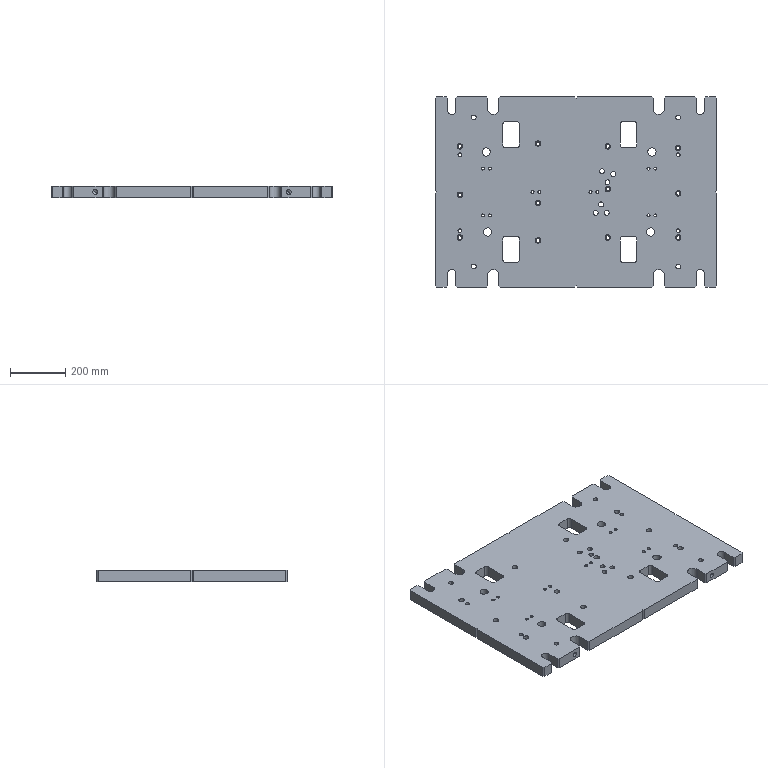Part | CATIA | 1 solid | 254 faces | box 1020 x 690 x 40 mm | volume 26113969 mm3 | cylinder 148 | plane 90 | cone 16 | commonest cylinder face diameters 20 x40 11 x24 13 x24 17.5 x16 18 x12 30 x12